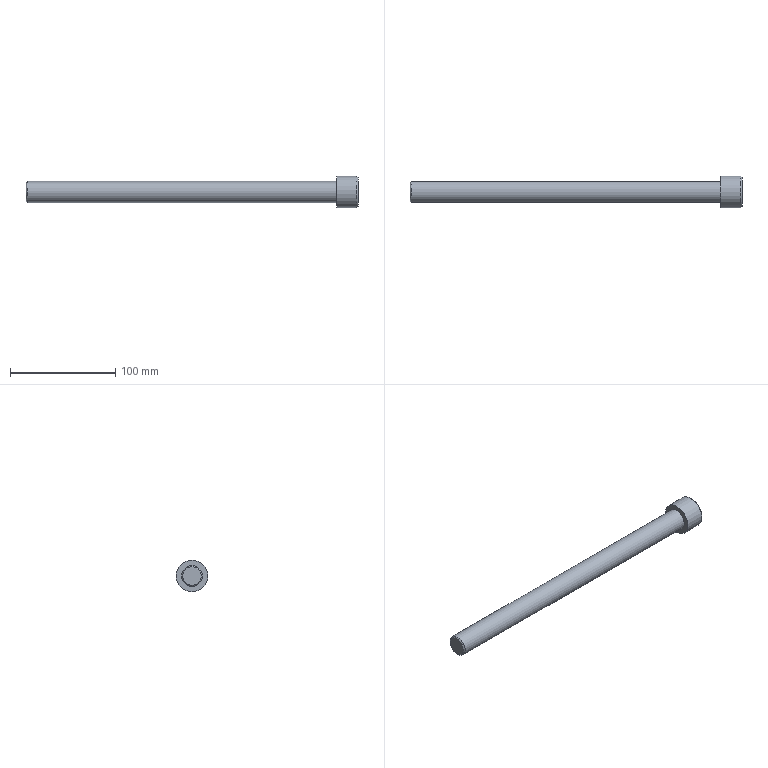Part | STEP file | solid 259 | 1 solid | 14 faces | box 315 x 30 x 30 mm | volume 103942 mm3 | plane 10 | cylinder 2 | cone 2 | commonest cylinder face diameters 20 x1 30 x1